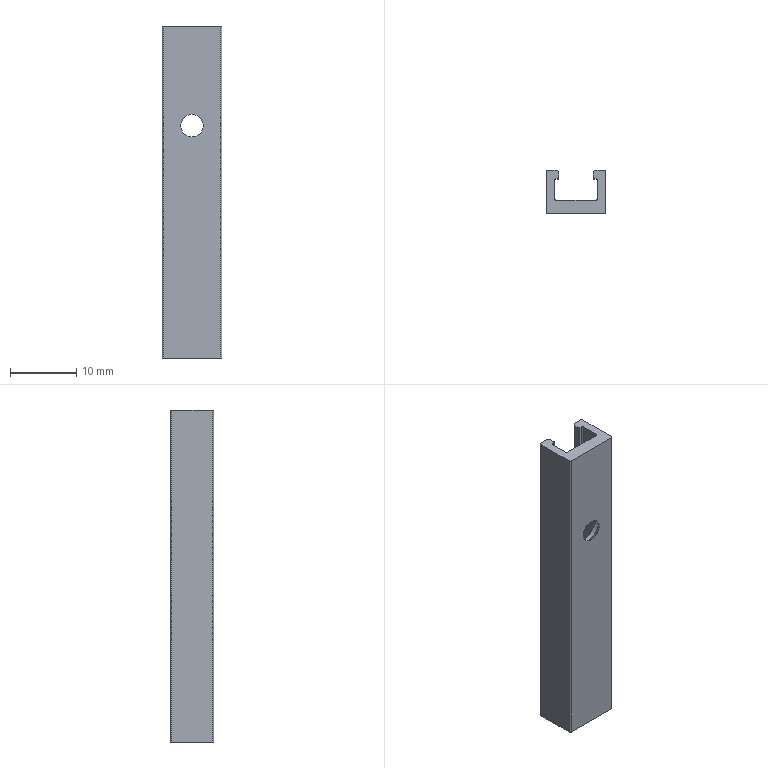Part | STEP file | 1 solid | 28 faces | box 9 x 6.5 x 50 mm | volume 1500 mm3 | plane 14 | cylinder 13 | cone 1 | commonest cylinder face diameters 0.4 x10 0.8 x2 6 x1